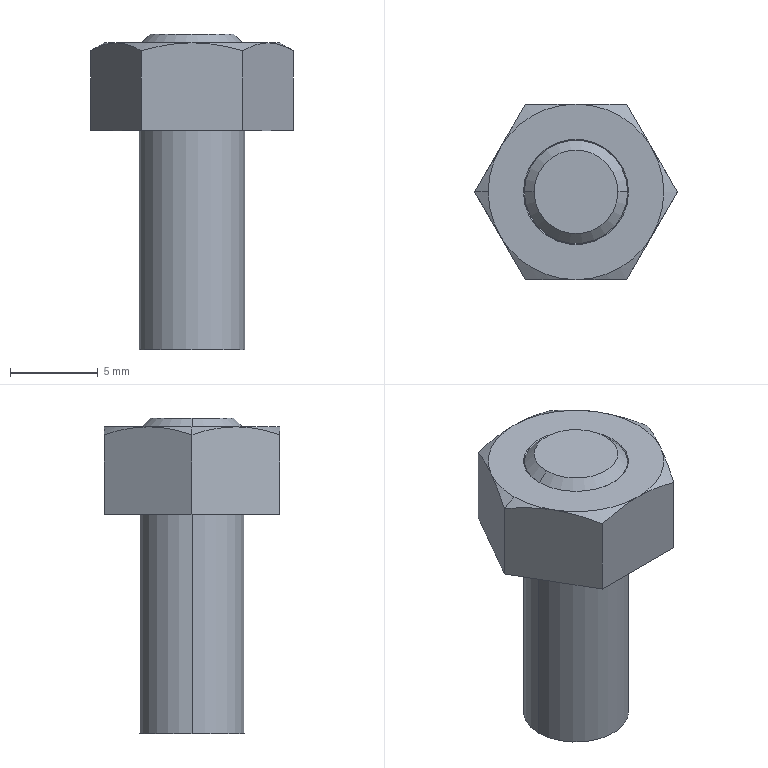Part | STEP file | ASND-0110-Q20 | 1 solid | 30 faces | box 11.547 x 10 x 18 mm | volume 731.296 mm3 | plane 17 | cone 11 | cylinder 2 | commonest cylinder face diameters 6 x2